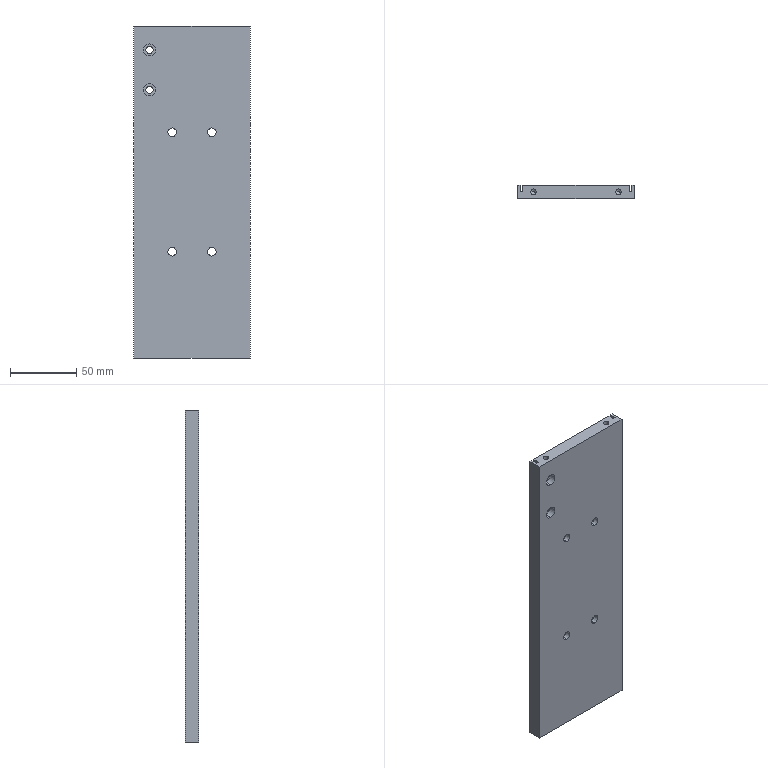Part | SolidWorks | features ICE 5, 3DProfileFeature 2, HoleWzd 2, Extrusion 1 | 1 solid | 60 faces | box 88 x 10 x 250 mm | volume 210737 mm3 | cylinder 32 | plane 20 | cone 8 | commonest cylinder face diameters 4.2 x8 6.5 x8 11 x8 5.5 x4 9 x4